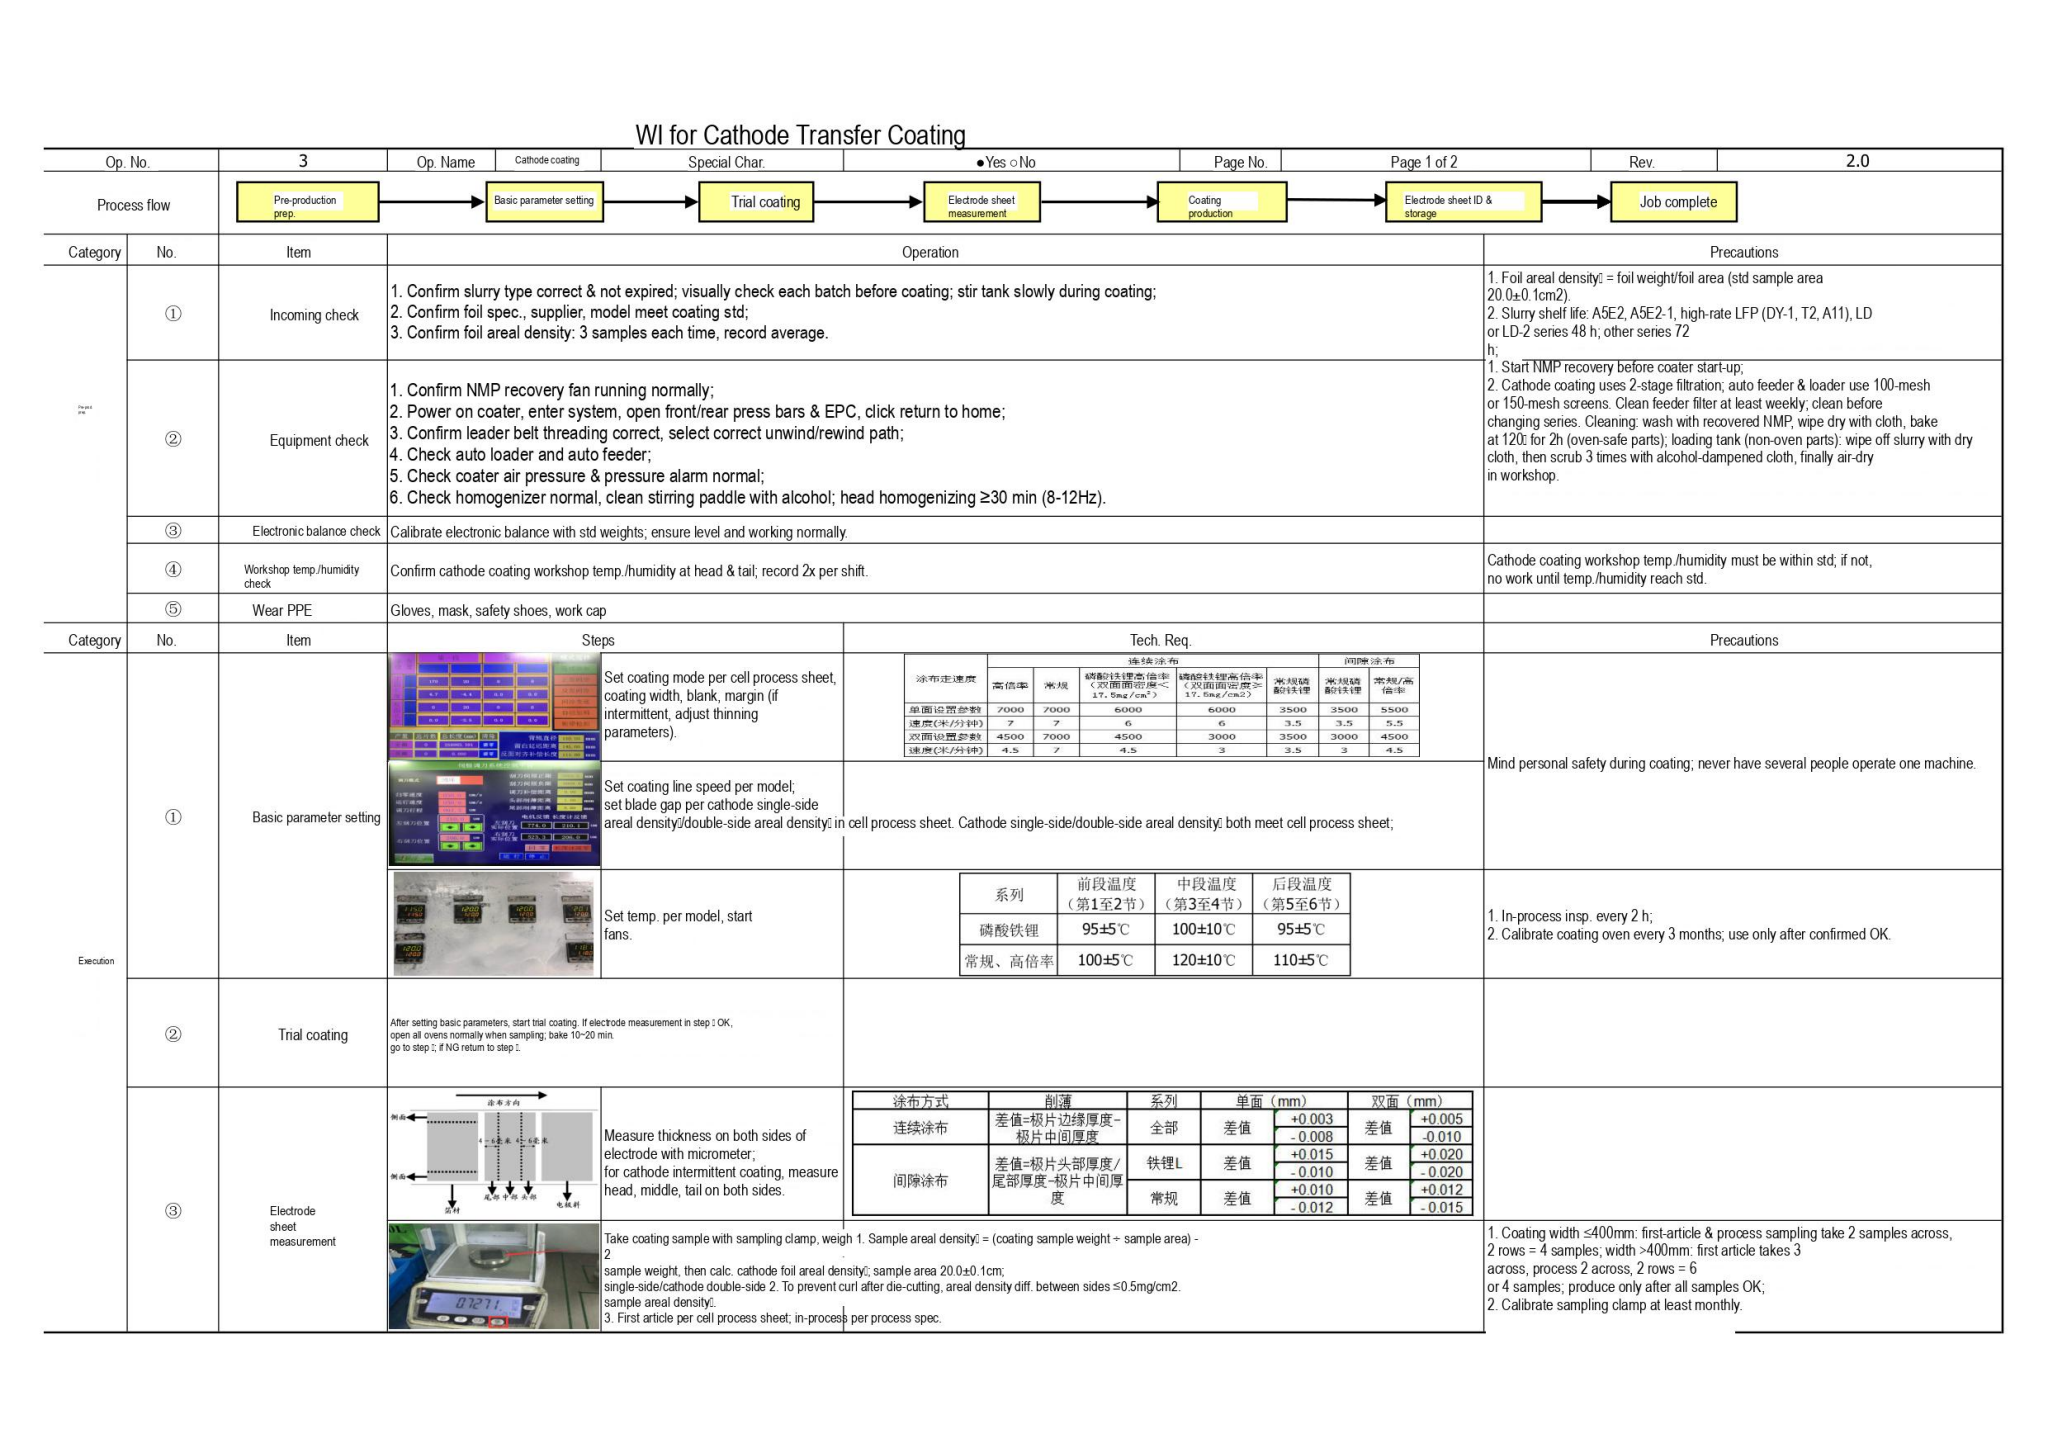# WI for Cathode Transfer Coating

| Op. No. | 3 | Op. Name | Cathode coating | Special Char. | ●Yes ○No | Page No. | Page 1 of 2 | Rev. | 2.0 |
|---|---|---|---|---|---|---|---|---|---|

**Process flow:** Pre-production prep. → Basic parameter setting → Trial coating → Electrode sheet measurement → Coating production → Electrode sheet ID & storage → Job complete

| Category | No. | Item | Operation | Precautions |
|---|---|---|---|---|
| | ① | Incoming check | 1. Confirm slurry type correct & not expired; visually check each batch before coating; stir tank slowly during coating;<br>2. Confirm foil spec., supplier, model meet coating std;<br>3. Confirm foil areal density: 3 samples each time, record average. | 1. Foil areal density = foil weight/foil area (std sample area 20.0±0.1cm2).<br>2. Slurry shelf life: A5E2, A5E2-1, high-rate LFP (DY-1, T2, A11), LD or LD-2 series 48 h; other series 72 h; |
| | ② | Equipment check | 1. Confirm NMP recovery fan running normally;<br>2. Power on coater, enter system, open front/rear press bars & EPC, click return to home;<br>3. Confirm leader belt threading correct, select correct unwind/rewind path;<br>4. Check auto loader and auto feeder;<br>5. Check coater air pressure & pressure alarm normal;<br>6. Check homogenizer normal, clean stirring paddle with alcohol; head homogenizing ≥30 min (8-12Hz). | 1. Start NMP recovery before coater start-up;<br>2. Cathode coating uses 2-stage filtration; auto feeder & loader use 100-mesh or 150-mesh screens. Clean feeder filter at least weekly; clean before changing series. Cleaning: wash with recovered NMP, wipe dry with cloth, bake at 120 for 2h (oven-safe parts); loading tank (non-oven parts): wipe off slurry with dry cloth, then scrub 3 times with alcohol-dampened cloth, finally air-dry in workshop. |
| | ③ | Electronic balance check | Calibrate electronic balance with std weights; ensure level and working normally. | |
| | ④ | Workshop temp./humidity check | Confirm cathode coating workshop temp./humidity at head & tail; record 2x per shift. | Cathode coating workshop temp./humidity must be within std; if not, no work until temp./humidity reach std. |
| | ⑤ | Wear PPE | Gloves, mask, safety shoes, work cap | |

| Category | No. | Item | Steps | Tech. Req. | Precautions |
|---|---|---|---|---|---|
| Execution | ① | Basic parameter setting | Set coating mode per cell process sheet, coating width, blank, margin (if intermittent, adjust thinning parameters). | (see table A) | Mind personal safety during coating; never have several people operate one machine. |
| | | | Set coating line speed per model; set blade gap per cathode single-side areal density/double-side areal density in cell process sheet. Cathode single-side/double-side areal density both meet cell process sheet; | | |
| | | | Set temp. per model, start fans. | (see table B) | 1. In-process insp. every 2 h;<br>2. Calibrate coating oven every 3 months; use only after confirmed OK. |
| | ② | Trial coating | After setting basic parameters, start trial coating. If electrode measurement in step OK, open all ovens normally when sampling; bake 10~20 min. go to step ; if NG return to step . | | |
| | ③ | Electrode sheet measurement | Measure thickness on both sides of electrode with micrometer; for cathode intermittent coating, measure head, middle, tail on both sides. | (see table C) | |
| | | | Take coating sample with sampling clamp, weigh sample weight, then calc. cathode foil areal density; sample area 20.0±0.1cm; single-side/cathode double-side sample areal density. | 1. Sample areal density = (coating sample weight ÷ sample area) -<br>2. To prevent curl after die-cutting, areal density diff. between sides ≤0.5mg/cm2.<br>3. First article per cell process sheet; in-process per process spec. | 1. Coating width ≤400mm: first-article & process sampling take 2 samples across, 2 rows = 4 samples; width >400mm: first article takes 3 across, process 2 across, 2 rows = 6 or 4 samples; produce only after all samples OK;<br>2. Calibrate sampling clamp at least monthly. |

Table A

| 涂布走速度 | 连续涂布<br>高倍率 | 连续涂布<br>常规 | 连续涂布<br>磷酸铁锂高倍率（双面面密度<17.5mg/cm²） | 连续涂布<br>磷酸铁锂高倍率（双面面密度≥17.5mg/cm2） | 连续涂布<br>常规磷酸铁锂 | 间隙涂布<br>常规磷酸铁锂 | 间隙涂布<br>常规/高倍率 |
|---|---|---|---|---|---|---|---|
| 单面设置参数 | 7000 | 7000 | 6000 | 6000 | 3500 | 3500 | 5500 |
| 速度(米/分钟) | 7 | 7 | 6 | 6 | 3.5 | 3.5 | 5.5 |
| 双面设置参数 | 4500 | 7000 | 4500 | 3000 | 3500 | 3000 | 4500 |
| 速度(米/分钟) | 4.5 | 7 | 4.5 | 3 | 3.5 | 3 | 4.5 |

Table B

| 系列 | 前段温度（第1至2节） | 中段温度（第3至4节） | 后段温度（第5至6节） |
|---|---|---|---|
| 磷酸铁锂 | 95±5℃ | 100±10℃ | 95±5℃ |
| 常规、高倍率 | 100±5℃ | 120±10℃ | 110±5℃ |

Table C

| 涂布方式 | 削薄 | 系列 | 单面（mm） | | 双面（mm） | |
|---|---|---|---|---|---|---|
| 连续涂布 | 差值=极片边缘厚度-极片中间厚度 | 全部 | 差值 | +0.003<br>-0.008 | 差值 | +0.005<br>-0.010 |
| 间隙涂布 | 差值=极片头部厚度/尾部厚度-极片中间厚度 | 铁锂L | 差值 | +0.015<br>-0.010 | 差值 | +0.020<br>-0.020 |
| | | 常规 | 差值 | +0.010<br>-0.012 | 差值 | +0.012<br>-0.015 |

涂布方向
侧面
侧面
4-6毫米 4-6毫米
尾部 中部 头部
箔材
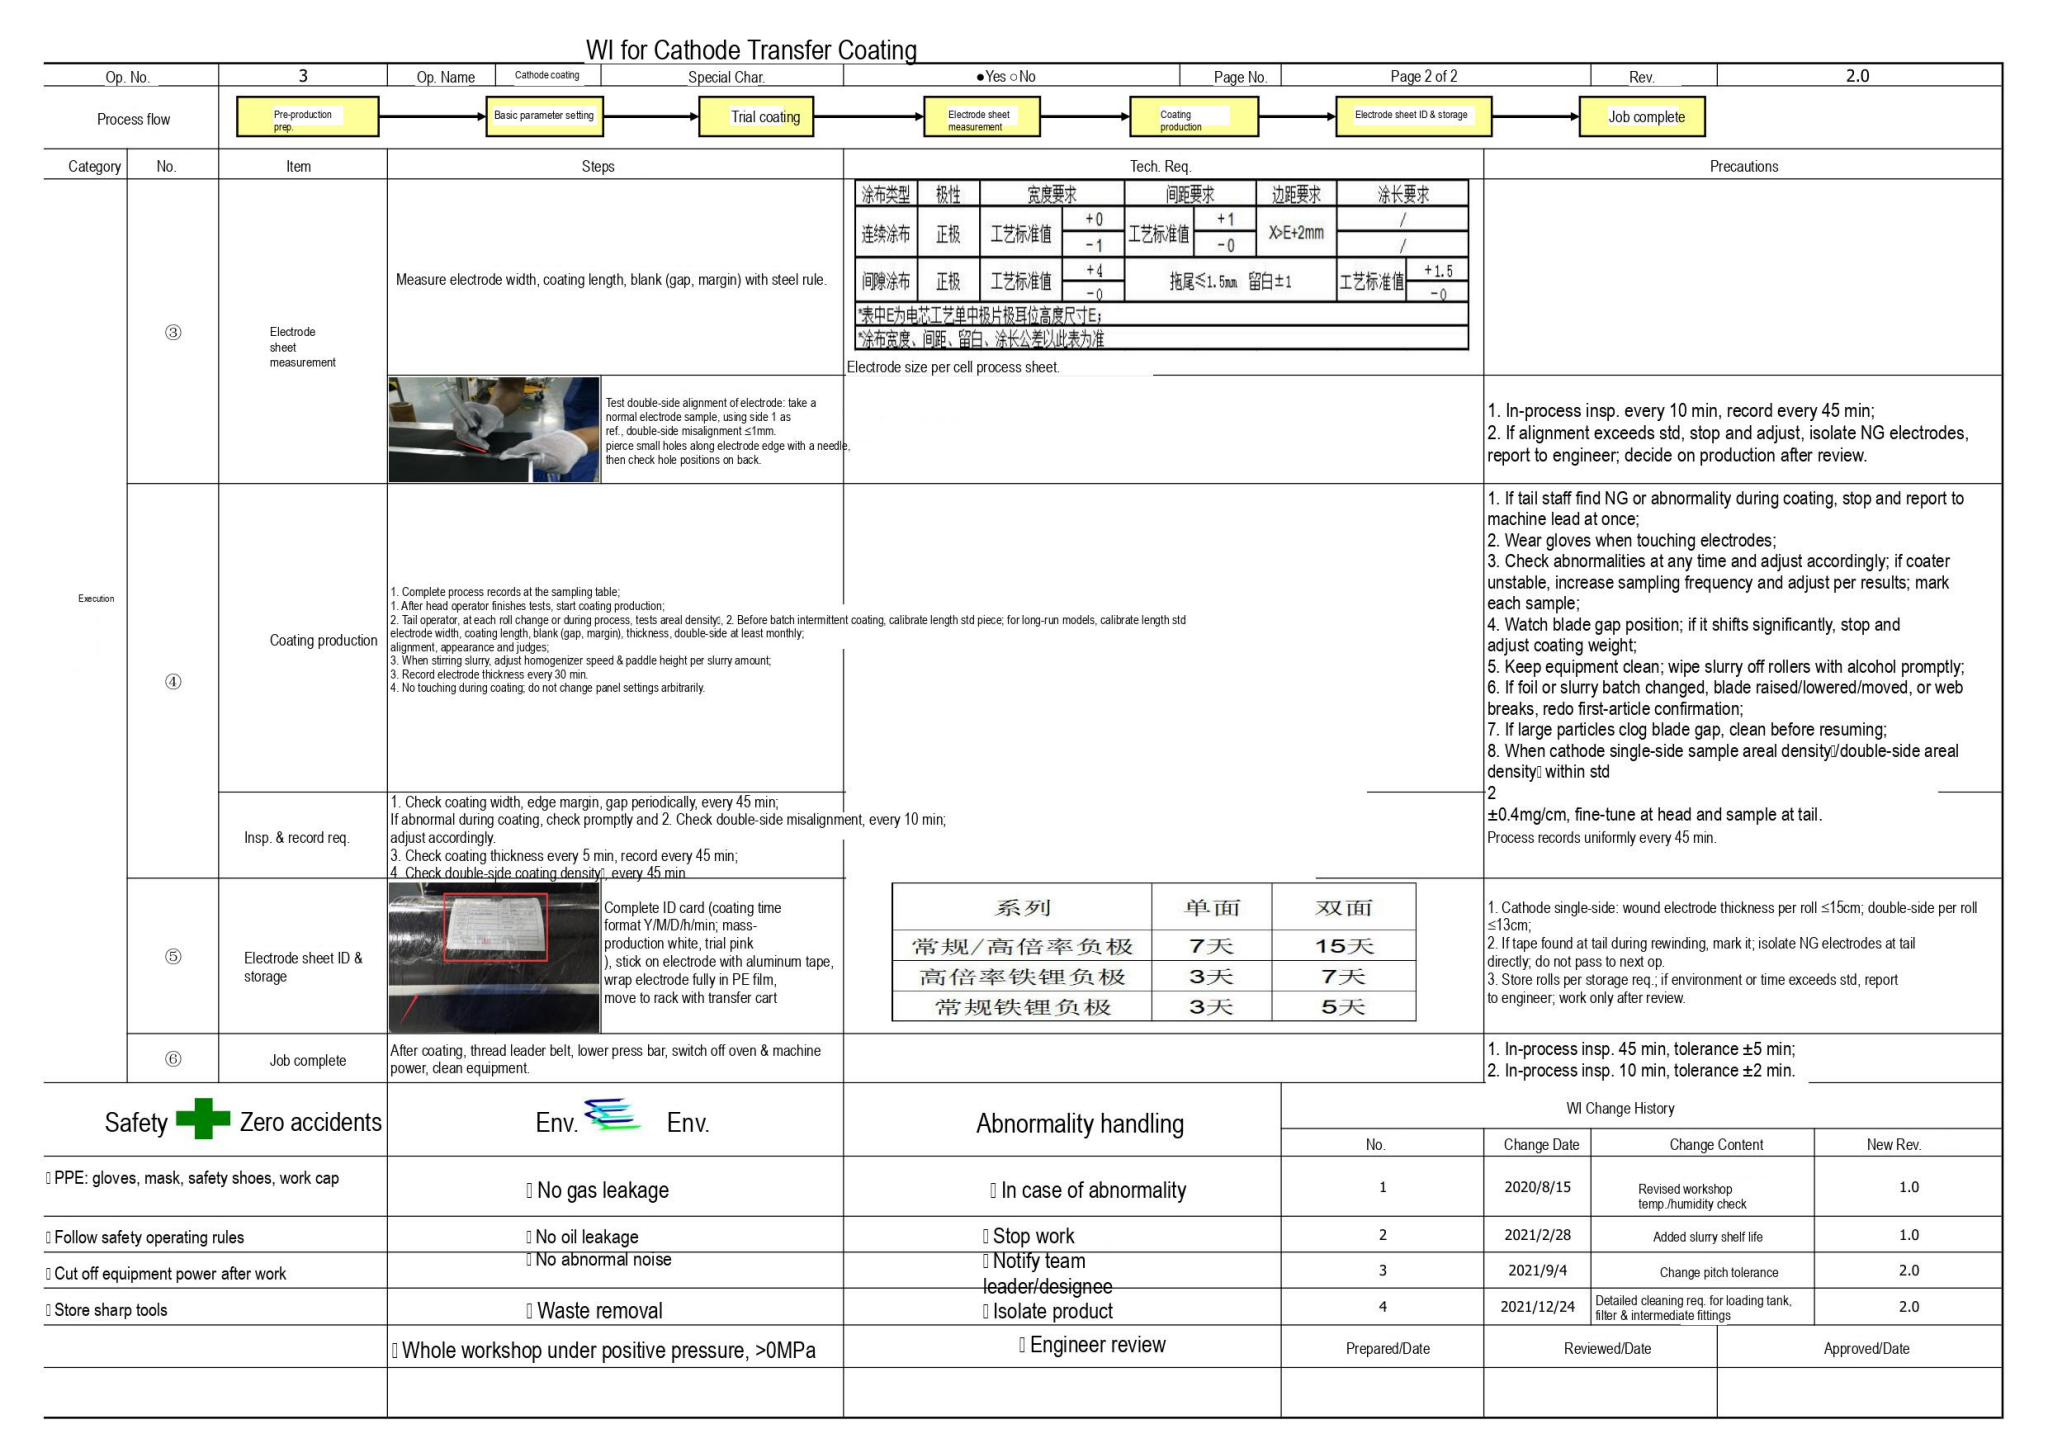# WI for Cathode Transfer Coating

| Op. No. | 3 | Op. Name | Cathode coating | Special Char. | ●Yes ○No | Page No. | Page 2 of 2 | Rev. | 2.0 |
|---|---|---|---|---|---|---|---|---|---|

| Process flow | Pre-production prep. → Basic parameter setting → Trial coating → Electrode sheet measurement → Coating production → Electrode sheet ID & storage → Job complete |
|---|---|

| Category | No. | Item | Steps | Tech. Req. | Precautions |
|---|---|---|---|---|---|
| Execution | ③ | Electrode sheet measurement | Measure electrode width, coating length, blank (gap, margin) with steel rule. | (see table A below) Electrode size per cell process sheet. | |
| | | | Test double-side alignment of electrode: take a normal electrode sample, using side 1 as ref., double-side misalignment ≤1mm. pierce small holes along electrode edge with a needle, then check hole positions on back. | | 1. In-process insp. every 10 min, record every 45 min;<br>2. If alignment exceeds std, stop and adjust, isolate NG electrodes, report to engineer; decide on production after review. |
| | ④ | Coating production | 1. Complete process records at the sampling table;<br>1. After head operator finishes tests, start coating production;<br>2. Tail operator, at each roll change or during process, tests areal density, 2. Before batch intermittent coating, calibrate length std piece; for long-run models, calibrate length std electrode width, coating length, blank (gap, margin), thickness, double-side at least monthly;<br>alignment, appearance and judges;<br>3. When stirring slurry, adjust homogenizer speed & paddle height per slurry amount;<br>3. Record electrode thickness every 30 min.<br>4. No touching during coating; do not change panel settings arbitrarily. | | 1. If tail staff find NG or abnormality during coating, stop and report to machine lead at once;<br>2. Wear gloves when touching electrodes;<br>3. Check abnormalities at any time and adjust accordingly; if coater unstable, increase sampling frequency and adjust per results; mark each sample;<br>4. Watch blade gap position; if it shifts significantly, stop and adjust coating weight;<br>5. Keep equipment clean; wipe slurry off rollers with alcohol promptly;<br>6. If foil or slurry batch changed, blade raised/lowered/moved, or web breaks, redo first-article confirmation;<br>7. If large particles clog blade gap, clean before resuming;<br>8. When cathode single-side sample areal density/double-side areal density within std<br>2<br>±0.4mg/cm, fine-tune at head and sample at tail. |
| | | Insp. & record req. | 1. Check coating width, edge margin, gap periodically, every 45 min;<br>If abnormal during coating, check promptly and 2. Check double-side misalignment, every 10 min; adjust accordingly.<br>3. Check coating thickness every 5 min, record every 45 min;<br>4. Check double-side coating density, every 45 min | | Process records uniformly every 45 min. |
| | ⑤ | Electrode sheet ID & storage | Complete ID card (coating time format Y/M/D/h/min; mass-production white, trial pink ), stick on electrode with aluminum tape, wrap electrode fully in PE film, move to rack with transfer cart | (see table B below) | 1. Cathode single-side: wound electrode thickness per roll ≤15cm; double-side per roll ≤13cm;<br>2. If tape found at tail during rewinding, mark it; isolate NG electrodes at tail directly; do not pass to next op.<br>3. Store rolls per storage req.; if environment or time exceeds std, report to engineer; work only after review. |
| | ⑥ | Job complete | After coating, thread leader belt, lower press bar, switch off oven & machine power, clean equipment. | | 1. In-process insp. 45 min, tolerance ±5 min;<br>2. In-process insp. 10 min, tolerance ±2 min. |

Table A (Tech. Req. ③):

| 涂布类型 | 极性 | 宽度要求 | | 间距要求 | | 边距要求 | 涂长要求 | |
|---|---|---|---|---|---|---|---|---|
| 连续涂布 | 正极 | 工艺标准值 | +0 / -1 | 工艺标准值 | +1 / -0 | X>E+2mm | / | / |
| 间隙涂布 | 正极 | 工艺标准值 | +4 / -0 | 拖尾≤1.5mm 留白±1 | | | 工艺标准值 | +1.5 / -0 |

*表中E为电芯工艺单中极片极耳位高度尺寸E;
*涂布宽度、间距、留白、涂长公差以此表为准

Table B (Tech. Req. ⑤):

| 系列 | 单面 | 双面 |
|---|---|---|
| 常规/高倍率负极 | 7天 | 15天 |
| 高倍率铁锂负极 | 3天 | 7天 |
| 常规铁锂负极 | 3天 | 5天 |

| Safety Zero accidents | Env. Env. | Abnormality handling |
|---|---|---|
| PPE: gloves, mask, safety shoes, work cap | No gas leakage | In case of abnormality |
| Follow safety operating rules | No oil leakage | Stop work |
| Cut off equipment power after work | No abnormal noise | Notify team leader/designee |
| Store sharp tools | Waste removal | Isolate product |
| | Whole workshop under positive pressure, >0MPa | Engineer review |

WI Change History

| No. | Change Date | Change Content | New Rev. |
|---|---|---|---|
| 1 | 2020/8/15 | Revised workshop temp./humidity check | 1.0 |
| 2 | 2021/2/28 | Added slurry shelf life | 1.0 |
| 3 | 2021/9/4 | Change pitch tolerance | 2.0 |
| 4 | 2021/12/24 | Detailed cleaning req. for loading tank, filter & intermediate fittings | 2.0 |

| Prepared/Date | Reviewed/Date | Approved/Date |
|---|---|---|
| | | |